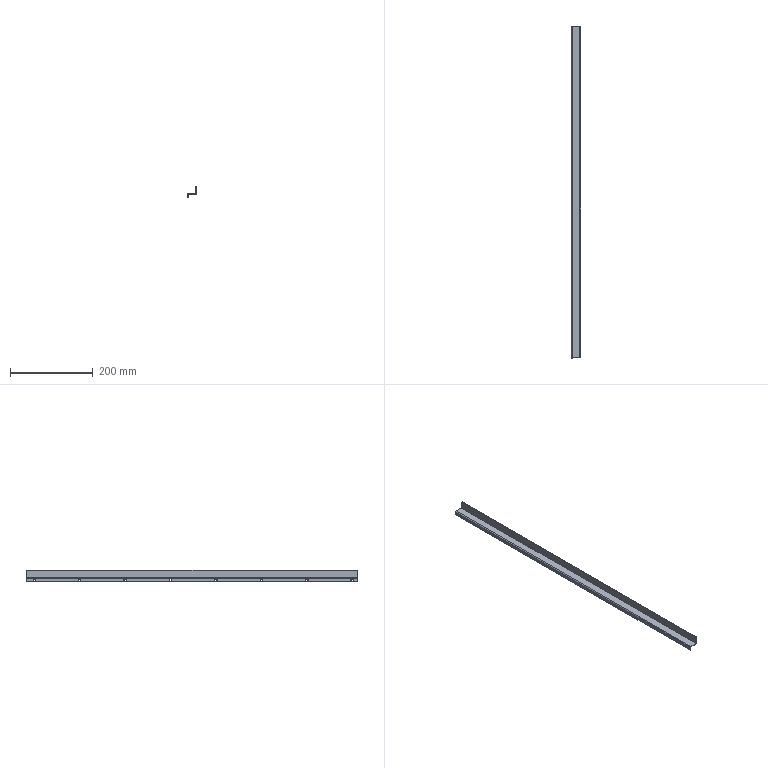Part | STEP file | Left Door Frame 1 | 1 solid | 38 faces | box 22 x 804 x 28 mm | volume 75069 mm3 | cylinder 22 | plane 16 | commonest cylinder face diameters 6 x16 0.2 x2 0.4 x2 4.2 x2
STEP:
#1=CARTESIAN_POINT('',(-10.939,692.193,-3.));
#2=VERTEX_POINT('',#1);
#3=CARTESIAN_POINT('',(-10.939,692.193,-9.));
#4=VERTEX_POINT('',#3);
#5=CARTESIAN_POINT('',(-10.939,692.193,-6.));
#6=DIRECTION('',(1.,0.,0.));
#7=DIRECTION('',(0.,0.,-1.));
#8=AXIS2_PLACEMENT_3D('',#5,#6,#7);
#9=CIRCLE('',#8,3.);
#10=EDGE_CURVE('',#2,#4,#9,.T.);
#11=ORIENTED_EDGE('',*,*,#10,.F.);
#12=CARTESIAN_POINT('',(-8.939,692.193,-3.));
#13=VERTEX_POINT('',#12);
#14=CARTESIAN_POINT('',(-18.939,692.193,-3.));
#15=DIRECTION('',(1.,0.,0.));
#16=VECTOR('',#15,1000.);
#17=LINE('',#14,#16);
#18=EDGE_CURVE('',#2,#13,#17,.T.);
#19=ORIENTED_EDGE('',*,*,#18,.T.);
#20=CARTESIAN_POINT('',(-8.939,692.193,-9.));
#21=VERTEX_POINT('',#20);
#22=CARTESIAN_POINT('',(-8.939,692.193,-6.));
#23=DIRECTION('',(-1.,0.,0.));
#24=DIRECTION('',(0.,0.,-1.));
#25=AXIS2_PLACEMENT_3D('',#22,#23,#24);
#26=CIRCLE('',#25,3.);
#27=EDGE_CURVE('',#21,#13,#26,.T.);
#28=ORIENTED_EDGE('',*,*,#27,.F.);
#29=CARTESIAN_POINT('',(-18.939,692.193,-9.));
#30=DIRECTION('',(1.,0.,0.));
#31=VECTOR('',#30,1000.);
#32=LINE('',#29,#31);
#33=EDGE_CURVE('',#4,#21,#32,.T.);
#34=ORIENTED_EDGE('',*,*,#33,.F.);
#35=EDGE_LOOP('',(#11,#19,#28,#34));
#36=FACE_OUTER_BOUND('',#35,.T.);
#37=CARTESIAN_POINT('',(-18.939,692.193,-6.));
#38=DIRECTION('',(1.,0.,0.));
#39=DIRECTION('',(0.,0.,-1.));
#40=AXIS2_PLACEMENT_3D('',#37,#38,#39);
#41=CYLINDRICAL_SURFACE('',#40,3.);
#42=ADVANCED_FACE('',(#36),#41,.F.);
#43=CARTESIAN_POINT('',(-10.939,582.193,-3.));
#44=VERTEX_POINT('',#43);
#45=CARTESIAN_POINT('',(-10.939,582.193,-9.));
#46=VERTEX_POINT('',#45);
#47=CARTESIAN_POINT('',(-10.939,582.193,-6.));
#48=DIRECTION('',(1.,0.,0.));
#49=DIRECTION('',(0.,0.,-1.));
#50=AXIS2_PLACEMENT_3D('',#47,#48,#49);
#51=CIRCLE('',#50,3.);
#52=EDGE_CURVE('',#44,#46,#51,.T.);
#53=ORIENTED_EDGE('',*,*,#52,.F.);
#54=CARTESIAN_POINT('',(-8.939,582.193,-3.));
#55=VERTEX_POINT('',#54);
#56=CARTESIAN_POINT('',(-18.939,582.193,-3.));
#57=DIRECTION('',(1.,0.,0.));
#58=VECTOR('',#57,1000.);
#59=LINE('',#56,#58);
#60=EDGE_CURVE('',#44,#55,#59,.T.);
#61=ORIENTED_EDGE('',*,*,#60,.T.);
#62=CARTESIAN_POINT('',(-8.939,582.193,-9.));
#63=VERTEX_POINT('',#62);
#64=CARTESIAN_POINT('',(-8.939,582.193,-6.));
#65=DIRECTION('',(-1.,0.,0.));
#66=DIRECTION('',(0.,0.,-1.));
#67=AXIS2_PLACEMENT_3D('',#64,#65,#66);
#68=CIRCLE('',#67,3.);
#69=EDGE_CURVE('',#63,#55,#68,.T.);
#70=ORIENTED_EDGE('',*,*,#69,.F.);
#71=CARTESIAN_POINT('',(-18.939,582.193,-9.));
#72=DIRECTION('',(1.,0.,0.));
#73=VECTOR('',#72,1000.);
#74=LINE('',#71,#73);
#75=EDGE_CURVE('',#46,#63,#74,.T.);
#76=ORIENTED_EDGE('',*,*,#75,.F.);
#77=EDGE_LOOP('',(#53,#61,#70,#76));
#78=FACE_OUTER_BOUND('',#77,.T.);
#79=CARTESIAN_POINT('',(-18.939,582.193,-6.));
#80=DIRECTION('',(1.,0.,0.));
#81=DIRECTION('',(0.,0.,-1.));
#82=AXIS2_PLACEMENT_3D('',#79,#80,#81);
#83=CYLINDRICAL_SURFACE('',#82,3.);
#84=ADVANCED_FACE('',(#78),#83,.F.);
#85=CARTESIAN_POINT('',(-10.939,472.193,-3.));
#86=VERTEX_POINT('',#85);
#87=CARTESIAN_POINT('',(-10.939,472.193,-9.));
#88=VERTEX_POINT('',#87);
#89=CARTESIAN_POINT('',(-10.939,472.193,-6.));
#90=DIRECTION('',(1.,0.,0.));
#91=DIRECTION('',(0.,0.,-1.));
#92=AXIS2_PLACEMENT_3D('',#89,#90,#91);
#93=CIRCLE('',#92,3.);
#94=EDGE_CURVE('',#86,#88,#93,.T.);
#95=ORIENTED_EDGE('',*,*,#94,.F.);
#96=CARTESIAN_POINT('',(-8.939,472.193,-3.));
#97=VERTEX_POINT('',#96);
#98=CARTESIAN_POINT('',(-18.939,472.193,-3.));
#99=DIRECTION('',(1.,0.,0.));
#100=VECTOR('',#99,1000.);
#101=LINE('',#98,#100);
#102=EDGE_CURVE('',#86,#97,#101,.T.);
#103=ORIENTED_EDGE('',*,*,#102,.T.);
#104=CARTESIAN_POINT('',(-8.939,472.193,-9.));
#105=VERTEX_POINT('',#104);
#106=CARTESIAN_POINT('',(-8.939,472.193,-6.));
#107=DIRECTION('',(-1.,0.,0.));
#108=DIRECTION('',(0.,0.,-1.));
#109=AXIS2_PLACEMENT_3D('',#106,#107,#108);
#110=CIRCLE('',#109,3.);
#111=EDGE_CURVE('',#105,#97,#110,.T.);
#112=ORIENTED_EDGE('',*,*,#111,.F.);
#113=CARTESIAN_POINT('',(-18.939,472.193,-9.));
#114=DIRECTION('',(1.,0.,0.));
#115=VECTOR('',#114,1000.);
#116=LINE('',#113,#115);
#117=EDGE_CURVE('',#88,#105,#116,.T.);
#118=ORIENTED_EDGE('',*,*,#117,.F.);
#119=EDGE_LOOP('',(#95,#103,#112,#118));
#120=FACE_OUTER_BOUND('',#119,.T.);
#121=CARTESIAN_POINT('',(-18.939,472.193,-6.));
#122=DIRECTION('',(1.,0.,0.));
#123=DIRECTION('',(0.,0.,-1.));
#124=AXIS2_PLACEMENT_3D('',#121,#122,#123);
#125=CYLINDRICAL_SURFACE('',#124,3.);
#126=ADVANCED_FACE('',(#120),#125,.F.);
#127=CARTESIAN_POINT('',(-10.939,362.193,-3.));
#128=VERTEX_POINT('',#127);
#129=CARTESIAN_POINT('',(-10.939,362.193,-9.));
#130=VERTEX_POINT('',#129);
#131=CARTESIAN_POINT('',(-10.939,362.193,-6.));
#132=DIRECTION('',(1.,0.,0.));
#133=DIRECTION('',(0.,0.,-1.));
#134=AXIS2_PLACEMENT_3D('',#131,#132,#133);
#135=CIRCLE('',#134,3.);
#136=EDGE_CURVE('',#128,#130,#135,.T.);
#137=ORIENTED_EDGE('',*,*,#136,.F.);
#138=CARTESIAN_POINT('',(-8.939,362.193,-3.));
#139=VERTEX_POINT('',#138);
#140=CARTESIAN_POINT('',(-18.939,362.193,-3.));
#141=DIRECTION('',(1.,0.,0.));
#142=VECTOR('',#141,1000.);
#143=LINE('',#140,#142);
#144=EDGE_CURVE('',#128,#139,#143,.T.);
#145=ORIENTED_EDGE('',*,*,#144,.T.);
#146=CARTESIAN_POINT('',(-8.939,362.193,-9.));
#147=VERTEX_POINT('',#146);
#148=CARTESIAN_POINT('',(-8.939,362.193,-6.));
#149=DIRECTION('',(-1.,0.,0.));
#150=DIRECTION('',(0.,0.,-1.));
#151=AXIS2_PLACEMENT_3D('',#148,#149,#150);
#152=CIRCLE('',#151,3.);
#153=EDGE_CURVE('',#147,#139,#152,.T.);
#154=ORIENTED_EDGE('',*,*,#153,.F.);
#155=CARTESIAN_POINT('',(-18.939,362.193,-9.));
#156=DIRECTION('',(1.,0.,0.));
#157=VECTOR('',#156,1000.);
#158=LINE('',#155,#157);
#159=EDGE_CURVE('',#130,#147,#158,.T.);
#160=ORIENTED_EDGE('',*,*,#159,.F.);
#161=EDGE_LOOP('',(#137,#145,#154,#160));
#162=FACE_OUTER_BOUND('',#161,.T.);
#163=CARTESIAN_POINT('',(-18.939,362.193,-6.));
#164=DIRECTION('',(1.,0.,0.));
#165=DIRECTION('',(0.,0.,-1.));
#166=AXIS2_PLACEMENT_3D('',#163,#164,#165);
#167=CYLINDRICAL_SURFACE('',#166,3.);
#168=ADVANCED_FACE('',(#162),#167,.F.);
#169=CARTESIAN_POINT('',(-10.939,252.193,-3.));
#170=VERTEX_POINT('',#169);
#171=CARTESIAN_POINT('',(-10.939,252.193,-9.));
#172=VERTEX_POINT('',#171);
#173=CARTESIAN_POINT('',(-10.939,252.193,-6.));
#174=DIRECTION('',(1.,0.,0.));
#175=DIRECTION('',(0.,0.,-1.));
#176=AXIS2_PLACEMENT_3D('',#173,#174,#175);
#177=CIRCLE('',#176,3.);
#178=EDGE_CURVE('',#170,#172,#177,.T.);
#179=ORIENTED_EDGE('',*,*,#178,.F.);
#180=CARTESIAN_POINT('',(-8.939,252.193,-3.));
#181=VERTEX_POINT('',#180);
#182=CARTESIAN_POINT('',(-18.939,252.193,-3.));
#183=DIRECTION('',(1.,0.,0.));
#184=VECTOR('',#183,1000.);
#185=LINE('',#182,#184);
#186=EDGE_CURVE('',#170,#181,#185,.T.);
#187=ORIENTED_EDGE('',*,*,#186,.T.);
#188=CARTESIAN_POINT('',(-8.939,252.193,-9.));
#189=VERTEX_POINT('',#188);
#190=CARTESIAN_POINT('',(-8.939,252.193,-6.));
#191=DIRECTION('',(-1.,0.,0.));
#192=DIRECTION('',(0.,0.,-1.));
#193=AXIS2_PLACEMENT_3D('',#190,#191,#192);
#194=CIRCLE('',#193,3.);
#195=EDGE_CURVE('',#189,#181,#194,.T.);
#196=ORIENTED_EDGE('',*,*,#195,.F.);
#197=CARTESIAN_POINT('',(-18.939,252.193,-9.));
#198=DIRECTION('',(1.,0.,0.));
#199=VECTOR('',#198,1000.);
#200=LINE('',#197,#199);
#201=EDGE_CURVE('',#172,#189,#200,.T.);
#202=ORIENTED_EDGE('',*,*,#201,.F.);
#203=EDGE_LOOP('',(#179,#187,#196,#202));
#204=FACE_OUTER_BOUND('',#203,.T.);
#205=CARTESIAN_POINT('',(-18.939,252.193,-6.));
#206=DIRECTION('',(1.,0.,0.));
#207=DIRECTION('',(0.,0.,-1.));
#208=AXIS2_PLACEMENT_3D('',#205,#206,#207);
#209=CYLINDRICAL_SURFACE('',#208,3.);
#210=ADVANCED_FACE('',(#204),#209,.F.);
#211=CARTESIAN_POINT('',(-10.939,142.193,-3.));
#212=VERTEX_POINT('',#211);
#213=CARTESIAN_POINT('',(-10.939,142.193,-9.));
#214=VERTEX_POINT('',#213);
#215=CARTESIAN_POINT('',(-10.939,142.193,-6.));
#216=DIRECTION('',(1.,0.,0.));
#217=DIRECTION('',(0.,0.,-1.));
#218=AXIS2_PLACEMENT_3D('',#215,#216,#217);
#219=CIRCLE('',#218,3.);
#220=EDGE_CURVE('',#212,#214,#219,.T.);
#221=ORIENTED_EDGE('',*,*,#220,.F.);
#222=CARTESIAN_POINT('',(-8.939,142.193,-3.));
#223=VERTEX_POINT('',#222);
#224=CARTESIAN_POINT('',(-18.939,142.193,-3.));
#225=DIRECTION('',(1.,0.,0.));
#226=VECTOR('',#225,1000.);
#227=LINE('',#224,#226);
#228=EDGE_CURVE('',#212,#223,#227,.T.);
#229=ORIENTED_EDGE('',*,*,#228,.T.);
#230=CARTESIAN_POINT('',(-8.939,142.193,-9.));
#231=VERTEX_POINT('',#230);
#232=CARTESIAN_POINT('',(-8.939,142.193,-6.));
#233=DIRECTION('',(-1.,0.,0.));
#234=DIRECTION('',(0.,0.,-1.));
#235=AXIS2_PLACEMENT_3D('',#232,#233,#234);
#236=CIRCLE('',#235,3.);
#237=EDGE_CURVE('',#231,#223,#236,.T.);
#238=ORIENTED_EDGE('',*,*,#237,.F.);
#239=CARTESIAN_POINT('',(-18.939,142.193,-9.));
#240=DIRECTION('',(1.,0.,0.));
#241=VECTOR('',#240,1000.);
#242=LINE('',#239,#241);
#243=EDGE_CURVE('',#214,#231,#242,.T.);
#244=ORIENTED_EDGE('',*,*,#243,.F.);
#245=EDGE_LOOP('',(#221,#229,#238,#244));
#246=FACE_OUTER_BOUND('',#245,.T.);
#247=CARTESIAN_POINT('',(-18.939,142.193,-6.));
#248=DIRECTION('',(1.,0.,0.));
#249=DIRECTION('',(0.,0.,-1.));
#250=AXIS2_PLACEMENT_3D('',#247,#248,#249);
#251=CYLINDRICAL_SURFACE('',#250,3.);
#252=ADVANCED_FACE('',(#246),#251,.F.);
#253=CARTESIAN_POINT('',(-10.939,32.193,-3.));
#254=VERTEX_POINT('',#253);
#255=CARTESIAN_POINT('',(-10.939,32.193,-9.));
#256=VERTEX_POINT('',#255);
#257=CARTESIAN_POINT('',(-10.939,32.193,-6.));
#258=DIRECTION('',(1.,0.,0.));
#259=DIRECTION('',(0.,0.,-1.));
#260=AXIS2_PLACEMENT_3D('',#257,#258,#259);
#261=CIRCLE('',#260,3.);
#262=EDGE_CURVE('',#254,#256,#261,.T.);
#263=ORIENTED_EDGE('',*,*,#262,.F.);
#264=CARTESIAN_POINT('',(-8.939,32.193,-3.));
#265=VERTEX_POINT('',#264);
#266=CARTESIAN_POINT('',(-18.939,32.193,-3.));
#267=DIRECTION('',(1.,0.,0.));
#268=VECTOR('',#267,1000.);
#269=LINE('',#266,#268);
#270=EDGE_CURVE('',#254,#265,#269,.T.);
#271=ORIENTED_EDGE('',*,*,#270,.T.);
#272=CARTESIAN_POINT('',(-8.939,32.193,-9.));
#273=VERTEX_POINT('',#272);
#274=CARTESIAN_POINT('',(-8.939,32.193,-6.));
#275=DIRECTION('',(-1.,0.,0.));
#276=DIRECTION('',(0.,0.,-1.));
#277=AXIS2_PLACEMENT_3D('',#274,#275,#276);
#278=CIRCLE('',#277,3.);
#279=EDGE_CURVE('',#273,#265,#278,.T.);
#280=ORIENTED_EDGE('',*,*,#279,.F.);
#281=CARTESIAN_POINT('',(-18.939,32.193,-9.));
#282=DIRECTION('',(1.,0.,0.));
#283=VECTOR('',#282,1000.);
#284=LINE('',#281,#283);
#285=EDGE_CURVE('',#256,#273,#284,.T.);
#286=ORIENTED_EDGE('',*,*,#285,.F.);
#287=EDGE_LOOP('',(#263,#271,#280,#286));
#288=FACE_OUTER_BOUND('',#287,.T.);
#289=CARTESIAN_POINT('',(-18.939,32.193,-6.));
#290=DIRECTION('',(1.,0.,0.));
#291=DIRECTION('',(0.,0.,-1.));
#292=AXIS2_PLACEMENT_3D('',#289,#290,#291);
#293=CYLINDRICAL_SURFACE('',#292,3.);
#294=ADVANCED_FACE('',(#288),#293,.F.);
#295=CARTESIAN_POINT('',(-10.939,-77.807,-3.));
#296=VERTEX_POINT('',#295);
#297=CARTESIAN_POINT('',(-10.939,-77.807,-9.));
#298=VERTEX_POINT('',#297);
#299=CARTESIAN_POINT('',(-10.939,-77.807,-6.));
#300=DIRECTION('',(1.,0.,0.));
#301=DIRECTION('',(0.,0.,-1.));
#302=AXIS2_PLACEMENT_3D('',#299,#300,#301);
#303=CIRCLE('',#302,3.);
#304=EDGE_CURVE('',#296,#298,#303,.T.);
#305=ORIENTED_EDGE('',*,*,#304,.F.);
#306=CARTESIAN_POINT('',(-8.939,-77.807,-3.));
#307=VERTEX_POINT('',#306);
#308=CARTESIAN_POINT('',(-18.939,-77.807,-3.));
#309=DIRECTION('',(1.,0.,0.));
#310=VECTOR('',#309,1000.);
#311=LINE('',#308,#310);
#312=EDGE_CURVE('',#296,#307,#311,.T.);
#313=ORIENTED_EDGE('',*,*,#312,.T.);
#314=CARTESIAN_POINT('',(-8.939,-77.807,-9.));
#315=VERTEX_POINT('',#314);
#316=CARTESIAN_POINT('',(-8.939,-77.807,-6.));
#317=DIRECTION('',(-1.,0.,0.));
#318=DIRECTION('',(0.,0.,-1.));
#319=AXIS2_PLACEMENT_3D('',#316,#317,#318);
#320=CIRCLE('',#319,3.);
#321=EDGE_CURVE('',#315,#307,#320,.T.);
#322=ORIENTED_EDGE('',*,*,#321,.F.);
#323=CARTESIAN_POINT('',(-18.939,-77.807,-9.));
#324=DIRECTION('',(1.,0.,0.));
#325=VECTOR('',#324,1000.);
#326=LINE('',#323,#325);
#327=EDGE_CURVE('',#298,#315,#326,.T.);
#328=ORIENTED_EDGE('',*,*,#327,.F.);
#329=EDGE_LOOP('',(#305,#313,#322,#328));
#330=FACE_OUTER_BOUND('',#329,.T.);
#331=CARTESIAN_POINT('',(-18.939,-77.807,-6.));
#332=DIRECTION('',(1.,0.,0.));
#333=DIRECTION('',(0.,0.,-1.));
#334=AXIS2_PLACEMENT_3D('',#331,#332,#333);
#335=CYLINDRICAL_SURFACE('',#334,3.);
#336=ADVANCED_FACE('',(#330),#335,.F.);
#337=CARTESIAN_POINT('',(9.061,-89.807,0.1));
#338=VERTEX_POINT('',#337);
#339=CARTESIAN_POINT('',(9.061,-89.807,18.));
#340=VERTEX_POINT('',#339);
#341=CARTESIAN_POINT('',(9.061,-89.807,0.));
#342=DIRECTION('',(0.,0.,1.));
#343=VECTOR('',#342,1000.);
#344=LINE('',#341,#343);
#345=EDGE_CURVE('',#338,#340,#344,.T.);
#346=ORIENTED_EDGE('',*,*,#345,.T.);
#347=CARTESIAN_POINT('',(9.061,710.193,18.));
#348=VERTEX_POINT('',#347);
#349=CARTESIAN_POINT('',(9.061,0.,18.));
#350=DIRECTION('',(0.,1.,0.));
#351=VECTOR('',#350,1000.);
#352=LINE('',#349,#351);
#353=EDGE_CURVE('',#340,#348,#352,.T.);
#354=ORIENTED_EDGE('',*,*,#353,.T.);
#355=CARTESIAN_POINT('',(9.061,710.193,0.1));
#356=VERTEX_POINT('',#355);
#357=CARTESIAN_POINT('',(9.061,710.193,0.));
#358=DIRECTION('',(0.,0.,-1.));
#359=VECTOR('',#358,1000.);
#360=LINE('',#357,#359);
#361=EDGE_CURVE('',#348,#356,#360,.T.);
#362=ORIENTED_EDGE('',*,*,#361,.T.);
#363=CARTESIAN_POINT('',(9.061,0.,0.1));
#364=DIRECTION('',(0.,-1.,0.));
#365=VECTOR('',#364,1000.);
#366=LINE('',#363,#365);
#367=EDGE_CURVE('',#356,#338,#366,.T.);
#368=ORIENTED_EDGE('',*,*,#367,.T.);
#369=EDGE_LOOP('',(#346,#354,#362,#368));
#370=FACE_OUTER_BOUND('',#369,.T.);
#371=CARTESIAN_POINT('',(9.061,0.,0.));
#372=DIRECTION('',(-1.,0.,0.));
#373=DIRECTION('',(0.,0.,1.));
#374=AXIS2_PLACEMENT_3D('',#371,#372,#373);
#375=PLANE('',#374);
#376=ADVANCED_FACE('',(#370),#375,.T.);
#377=CARTESIAN_POINT('',(11.061,-89.807,18.));
#378=VERTEX_POINT('',#377);
#379=CARTESIAN_POINT('',(11.061,-89.807,18.));
#380=DIRECTION('',(-1.,0.,0.));
#381=VECTOR('',#380,1000.);
#382=LINE('',#379,#381);
#383=EDGE_CURVE('',#378,#340,#382,.T.);
#384=ORIENTED_EDGE('',*,*,#383,.F.);
#385=CARTESIAN_POINT('',(11.061,710.193,18.));
#386=VERTEX_POINT('',#385);
#387=CARTESIAN_POINT('',(11.061,-89.807,18.));
#388=DIRECTION('',(0.,-1.,0.));
#389=VECTOR('',#388,1000.);
#390=LINE('',#387,#389);
#391=EDGE_CURVE('',#386,#378,#390,.T.);
#392=ORIENTED_EDGE('',*,*,#391,.F.);
#393=CARTESIAN_POINT('',(11.061,710.193,18.));
#394=DIRECTION('',(1.,0.,0.));
#395=VECTOR('',#394,1000.);
#396=LINE('',#393,#395);
#397=EDGE_CURVE('',#348,#386,#396,.T.);
#398=ORIENTED_EDGE('',*,*,#397,.F.);
#399=ORIENTED_EDGE('',*,*,#353,.F.);
#400=EDGE_LOOP('',(#384,#392,#398,#399));
#401=FACE_OUTER_BOUND('',#400,.T.);
#402=CARTESIAN_POINT('',(11.061,-89.807,18.));
#403=DIRECTION('',(0.,0.,-1.));
#404=DIRECTION('',(-1.,0.,0.));
#405=AXIS2_PLACEMENT_3D('',#402,#403,#404);
#406=PLANE('',#405);
#407=ADVANCED_FACE('',(#401),#406,.F.);
#408=CARTESIAN_POINT('',(11.061,-89.807,0.1));
#409=VERTEX_POINT('',#408);
#410=CARTESIAN_POINT('',(11.061,-89.807,0.));
#411=DIRECTION('',(0.,0.,-1.));
#412=VECTOR('',#411,1000.);
#413=LINE('',#410,#412);
#414=EDGE_CURVE('',#378,#409,#413,.T.);
#415=ORIENTED_EDGE('',*,*,#414,.F.);
#416=ORIENTED_EDGE('',*,*,#383,.T.);
#417=ORIENTED_EDGE('',*,*,#345,.F.);
#418=CARTESIAN_POINT('',(8.961,-89.807,0.));
#419=VERTEX_POINT('',#418);
#420=CARTESIAN_POINT('',(8.961,-89.807,0.1));
#421=DIRECTION('',(0.,1.,0.));
#422=DIRECTION('',(0.,0.,1.));
#423=AXIS2_PLACEMENT_3D('',#420,#421,#422);
#424=CIRCLE('',#423,0.1);
#425=EDGE_CURVE('',#338,#419,#424,.T.);
#426=ORIENTED_EDGE('',*,*,#425,.T.);
#427=CARTESIAN_POINT('',(8.561,-89.807,0.));
#428=VERTEX_POINT('',#427);
#429=CARTESIAN_POINT('',(0.,-89.807,0.));
#430=DIRECTION('',(1.,0.,0.));
#431=VECTOR('',#430,1000.);
#432=LINE('',#429,#431);
#433=EDGE_CURVE('',#428,#419,#432,.T.);
#434=ORIENTED_EDGE('',*,*,#433,.F.);
#435=CARTESIAN_POINT('',(8.561,-89.807,-2.));
#436=VERTEX_POINT('',#435);
#437=CARTESIAN_POINT('',(8.561,-89.807,0.));
#438=DIRECTION('',(0.,0.,-1.));
#439=VECTOR('',#438,1000.);
#440=LINE('',#437,#439);
#441=EDGE_CURVE('',#428,#436,#440,.T.);
#442=ORIENTED_EDGE('',*,*,#441,.T.);
#443=CARTESIAN_POINT('',(8.961,-89.807,-2.));
#444=VERTEX_POINT('',#443);
#445=CARTESIAN_POINT('',(8.961,-89.807,-2.));
#446=DIRECTION('',(1.,0.,0.));
#447=VECTOR('',#446,1000.);
#448=LINE('',#445,#447);
#449=EDGE_CURVE('',#436,#444,#448,.T.);
#450=ORIENTED_EDGE('',*,*,#449,.T.);
#451=CARTESIAN_POINT('',(8.961,-89.807,0.1));
#452=DIRECTION('',(0.,-1.,0.));
#453=DIRECTION('',(0.,0.,1.));
#454=AXIS2_PLACEMENT_3D('',#451,#452,#453);
#455=CIRCLE('',#454,2.1);
#456=EDGE_CURVE('',#444,#409,#455,.T.);
#457=ORIENTED_EDGE('',*,*,#456,.T.);
#458=EDGE_LOOP('',(#415,#416,#417,#426,#434,#442,#450,#457));
#459=FACE_OUTER_BOUND('',#458,.T.);
#460=CARTESIAN_POINT('',(11.061,-89.807,0.));
#461=DIRECTION('',(0.,1.,0.));
#462=DIRECTION('',(-1.,0.,0.));
#463=AXIS2_PLACEMENT_3D('',#460,#461,#462);
#464=PLANE('',#463);
#465=ADVANCED_FACE('',(#459),#464,.F.);
#466=ORIENTED_EDGE('',*,*,#425,.F.);
#467=ORIENTED_EDGE('',*,*,#367,.F.);
#468=CARTESIAN_POINT('',(8.961,710.193,0.));
#469=VERTEX_POINT('',#468);
#470=CARTESIAN_POINT('',(8.961,710.193,0.1));
#471=DIRECTION('',(0.,1.,0.));
#472=DIRECTION('',(0.,0.,1.));
#473=AXIS2_PLACEMENT_3D('',#470,#471,#472);
#474=CIRCLE('',#473,0.1);
#475=EDGE_CURVE('',#356,#469,#474,.T.);
#476=ORIENTED_EDGE('',*,*,#475,.T.);
#477=CARTESIAN_POINT('',(8.961,710.193,0.));
#478=DIRECTION('',(0.,1.,0.));
#479=VECTOR('',#478,1000.);
#480=LINE('',#477,#479);
#481=EDGE_CURVE('',#419,#469,#480,.T.);
#482=ORIENTED_EDGE('',*,*,#481,.F.);
#483=EDGE_LOOP('',(#466,#467,#476,#482));
#484=FACE_OUTER_BOUND('',#483,.T.);
#485=CARTESIAN_POINT('',(8.961,710.193,0.1));
#486=DIRECTION('',(0.,1.,0.));
#487=DIRECTION('',(0.,0.,1.));
#488=AXIS2_PLACEMENT_3D('',#485,#486,#487);
#489=CYLINDRICAL_SURFACE('',#488,0.1);
#490=ADVANCED_FACE('',(#484),#489,.F.);
#491=ORIENTED_EDGE('',*,*,#361,.F.);
#492=ORIENTED_EDGE('',*,*,#397,.T.);
#493=CARTESIAN_POINT('',(11.061,710.193,0.1));
#494=VERTEX_POINT('',#493);
#495=CARTESIAN_POINT('',(11.061,710.193,18.));
#496=DIRECTION('',(0.,0.,1.));
#497=VECTOR('',#496,1000.);
#498=LINE('',#495,#497);
#499=EDGE_CURVE('',#494,#386,#498,.T.);
#500=ORIENTED_EDGE('',*,*,#499,.F.);
#501=CARTESIAN_POINT('',(8.961,710.193,-2.));
#502=VERTEX_POINT('',#501);
#503=CARTESIAN_POINT('',(8.961,710.193,0.1));
#504=DIRECTION('',(0.,-1.,0.));
#505=DIRECTION('',(0.,0.,1.));
#506=AXIS2_PLACEMENT_3D('',#503,#504,#505);
#507=CIRCLE('',#506,2.1);
#508=EDGE_CURVE('',#502,#494,#507,.T.);
#509=ORIENTED_EDGE('',*,*,#508,.F.);
#510=CARTESIAN_POINT('',(8.561,710.193,-2.));
#511=VERTEX_POINT('',#510);
#512=CARTESIAN_POINT('',(8.561,710.193,-2.));
#513=DIRECTION('',(-1.,0.,0.));
#514=VECTOR('',#513,1000.);
#515=LINE('',#512,#514);
#516=EDGE_CURVE('',#502,#511,#515,.T.);
#517=ORIENTED_EDGE('',*,*,#516,.T.);
#518=CARTESIAN_POINT('',(8.561,710.193,0.));
#519=VERTEX_POINT('',#518);
#520=CARTESIAN_POINT('',(8.561,710.193,0.));
#521=DIRECTION('',(0.,0.,1.));
#522=VECTOR('',#521,1000.);
#523=LINE('',#520,#522);
#524=EDGE_CURVE('',#511,#519,#523,.T.);
#525=ORIENTED_EDGE('',*,*,#524,.T.);
#526=CARTESIAN_POINT('',(8.561,710.193,0.));
#527=DIRECTION('',(1.,0.,0.));
#528=VECTOR('',#527,1000.);
#529=LINE('',#526,#528);
#530=EDGE_CURVE('',#519,#469,#529,.T.);
#531=ORIENTED_EDGE('',*,*,#530,.T.);
#532=ORIENTED_EDGE('',*,*,#475,.F.);
#533=EDGE_LOOP('',(#491,#492,#500,#509,#517,#525,#531,#532));
#534=FACE_OUTER_BOUND('',#533,.T.);
#535=CARTESIAN_POINT('',(11.061,710.193,18.));
#536=DIRECTION('',(0.,-1.,0.));
#537=DIRECTION('',(1.,0.,0.));
#538=AXIS2_PLACEMENT_3D('',#535,#536,#537);
#539=PLANE('',#538);
#540=ADVANCED_FACE('',(#534),#539,.F.);
#541=ORIENTED_EDGE('',*,*,#499,.T.);
#542=ORIENTED_EDGE('',*,*,#391,.T.);
#543=ORIENTED_EDGE('',*,*,#414,.T.);
#544=CARTESIAN_POINT('',(11.061,0.,0.1));
#545=DIRECTION('',(0.,-1.,0.));
#546=VECTOR('',#545,1000.);
#547=LINE('',#544,#546);
#548=EDGE_CURVE('',#494,#409,#547,.T.);
#549=ORIENTED_EDGE('',*,*,#548,.F.);
#550=EDGE_LOOP('',(#541,#542,#543,#549));
#551=FACE_OUTER_BOUND('',#550,.T.);
#552=CARTESIAN_POINT('',(11.061,0.,0.));
#553=DIRECTION('',(-1.,0.,0.));
#554=DIRECTION('',(0.,0.,1.));
#555=AXIS2_PLACEMENT_3D('',#552,#553,#554);
#556=PLANE('',#555);
#557=ADVANCED_FACE('',(#551),#556,.F.);
#558=ORIENTED_EDGE('',*,*,#481,.T.);
#559=ORIENTED_EDGE('',*,*,#530,.F.);
#560=CARTESIAN_POINT('',(8.561,710.593,0.));
#561=VERTEX_POINT('',#560);
#562=CARTESIAN_POINT('',(8.561,710.393,0.));
#563=DIRECTION('',(0.,0.,-1.));
#564=DIRECTION('',(0.,1.,0.));
#565=AXIS2_PLACEMENT_3D('',#562,#563,#564);
#566=CIRCLE('',#565,0.2);
#567=EDGE_CURVE('',#519,#561,#566,.T.);
#568=ORIENTED_EDGE('',*,*,#567,.T.);
#569=CARTESIAN_POINT('',(11.061,710.593,0.));
#570=VERTEX_POINT('',#569);
#571=CARTESIAN_POINT('',(0.,710.593,0.));
#572=DIRECTION('',(1.,0.,0.));
#573=VECTOR('',#572,1000.);
#574=LINE('',#571,#573);
#575=EDGE_CURVE('',#561,#570,#574,.T.);
#576=ORIENTED_EDGE('',*,*,#575,.T.);
#577=CARTESIAN_POINT('',(11.061,712.193,0.));
#578=VERTEX_POINT('',#577);
#579=CARTESIAN_POINT('',(11.061,712.193,0.));
#580=DIRECTION('',(0.,-1.,0.));
#581=VECTOR('',#580,1000.);
#582=LINE('',#579,#581);
#583=EDGE_CURVE('',#578,#570,#582,.T.);
#584=ORIENTED_EDGE('',*,*,#583,.F.);
#585=CARTESIAN_POINT('',(-8.839,712.193,0.));
#586=VERTEX_POINT('',#585);
#587=CARTESIAN_POINT('',(0.,712.193,0.));
#588=DIRECTION('',(-1.,0.,0.));
#589=VECTOR('',#588,1000.);
#590=LINE('',#587,#589);
#591=EDGE_CURVE('',#578,#586,#590,.T.);
#592=ORIENTED_EDGE('',*,*,#591,.T.);
#593=CARTESIAN_POINT('',(-8.839,-91.807,0.));
#594=VERTEX_POINT('',#593);
#595=CARTESIAN_POINT('',(-8.839,0.,0.));
#596=DIRECTION('',(0.,-1.,0.));
#597=VECTOR('',#596,1000.);
#598=LINE('',#595,#597);
#599=EDGE_CURVE('',#586,#594,#598,.T.);
#600=ORIENTED_EDGE('',*,*,#599,.T.);
#601=CARTESIAN_POINT('',(11.061,-91.807,0.));
#602=VERTEX_POINT('',#601);
#603=CARTESIAN_POINT('',(0.,-91.807,0.));
#604=DIRECTION('',(1.,0.,0.));
#605=VECTOR('',#604,1000.);
#606=LINE('',#603,#605);
#607=EDGE_CURVE('',#594,#602,#606,.T.);
#608=ORIENTED_EDGE('',*,*,#607,.T.);
#609=CARTESIAN_POINT('',(11.061,-90.207,0.));
#610=VERTEX_POINT('',#609);
#611=CARTESIAN_POINT('',(11.061,712.193,0.));
#612=DIRECTION('',(0.,-1.,0.));
#613=VECTOR('',#612,1000.);
#614=LINE('',#611,#613);
#615=EDGE_CURVE('',#610,#602,#614,.T.);
#616=ORIENTED_EDGE('',*,*,#615,.F.);
#617=CARTESIAN_POINT('',(8.561,-90.207,0.));
#618=VERTEX_POINT('',#617);
#619=CARTESIAN_POINT('',(0.,-90.207,0.));
#620=DIRECTION('',(-1.,0.,0.));
#621=VECTOR('',#620,1000.);
#622=LINE('',#619,#621);
#623=EDGE_CURVE('',#610,#618,#622,.T.);
#624=ORIENTED_EDGE('',*,*,#623,.T.);
#625=CARTESIAN_POINT('',(8.561,-90.007,0.));
#626=DIRECTION('',(0.,0.,-1.));
#627=DIRECTION('',(0.,1.,0.));
#628=AXIS2_PLACEMENT_3D('',#625,#626,#627);
#629=CIRCLE('',#628,0.2);
#630=EDGE_CURVE('',#618,#428,#629,.T.);
#631=ORIENTED_EDGE('',*,*,#630,.T.);
#632=ORIENTED_EDGE('',*,*,#433,.T.);
#633=EDGE_LOOP('',(#558,#559,#568,#576,#584,#592,#600,#608,#616,#624,#631,#632));
#634=FACE_OUTER_BOUND('',#633,.T.);
#635=CARTESIAN_POINT('',(0.,0.,0.));
#636=DIRECTION('',(0.,0.,1.));
#637=DIRECTION('',(1.,0.,0.));
#638=AXIS2_PLACEMENT_3D('',#635,#636,#637);
#639=PLANE('',#638);
#640=ADVANCED_FACE('',(#634),#639,.T.);
#641=ORIENTED_EDGE('',*,*,#548,.T.);
#642=ORIENTED_EDGE('',*,*,#456,.F.);
#643=CARTESIAN_POINT('',(8.961,710.193,-2.));
#644=DIRECTION('',(0.,1.,0.));
#645=VECTOR('',#644,1000.);
#646=LINE('',#643,#645);
#647=EDGE_CURVE('',#444,#502,#646,.T.);
#648=ORIENTED_EDGE('',*,*,#647,.T.);
#649=ORIENTED_EDGE('',*,*,#508,.T.);
#650=EDGE_LOOP('',(#641,#642,#648,#649));
#651=FACE_OUTER_BOUND('',#650,.T.);
#652=CARTESIAN_POINT('',(8.961,710.193,0.1));
#653=DIRECTION('',(0.,1.,0.));
#654=DIRECTION('',(0.,0.,1.));
#655=AXIS2_PLACEMENT_3D('',#652,#653,#654);
#656=CYLINDRICAL_SURFACE('',#655,2.1);
#657=ADVANCED_FACE('',(#651),#656,.T.);
#658=CARTESIAN_POINT('',(8.561,-90.207,-2.));
#659=VERTEX_POINT('',#658);
#660=CARTESIAN_POINT('',(8.561,-90.207,0.));
#661=DIRECTION('',(0.,0.,1.));
#662=VECTOR('',#661,1000.);
#663=LINE('',#660,#662);
#664=EDGE_CURVE('',#659,#618,#663,.T.);
#665=ORIENTED_EDGE('',*,*,#664,.T.);
#666=ORIENTED_EDGE('',*,*,#623,.F.);
#667=CARTESIAN_POINT('',(11.061,-90.207,-2.));
#668=VERTEX_POINT('',#667);
#669=CARTESIAN_POINT('',(11.061,-90.207,0.));
#670=DIRECTION('',(0.,0.,-1.));
#671=VECTOR('',#670,1000.);
#672=LINE('',#669,#671);
#673=EDGE_CURVE('',#610,#668,#672,.T.);
#674=ORIENTED_EDGE('',*,*,#673,.T.);
#675=CARTESIAN_POINT('',(8.561,-90.207,-2.));
#676=DIRECTION('',(-1.,0.,0.));
#677=VECTOR('',#676,1000.);
#678=LINE('',#675,#677);
#679=EDGE_CURVE('',#668,#659,#678,.T.);
#680=ORIENTED_EDGE('',*,*,#679,.T.);
#681=EDGE_LOOP('',(#665,#666,#674,#680));
#682=FACE_OUTER_BOUND('',#681,.T.);
#683=CARTESIAN_POINT('',(8.561,-90.207,0.));
#684=DIRECTION('',(0.,1.,0.));
#685=DIRECTION('',(0.,0.,1.));
#686=AXIS2_PLACEMENT_3D('',#683,#684,#685);
#687=PLANE('',#686);
#688=ADVANCED_FACE('',(#682),#687,.T.);
#689=CARTESIAN_POINT('',(11.061,-91.807,-2.));
#690=VERTEX_POINT('',#689);
#691=CARTESIAN_POINT('',(11.061,-91.807,-2.));
#692=DIRECTION('',(0.,0.,1.));
#693=VECTOR('',#692,1000.);
#694=LINE('',#691,#693);
#695=EDGE_CURVE('',#690,#602,#694,.T.);
#696=ORIENTED_EDGE('',*,*,#695,.T.);
#697=ORIENTED_EDGE('',*,*,#607,.F.);
#698=CARTESIAN_POINT('',(-10.939,-91.807,-2.1));
#699=VERTEX_POINT('',#698);
#700=CARTESIAN_POINT('',(-8.839,-91.807,-2.1));
#701=DIRECTION('',(0.,1.,0.));
#702=DIRECTION('',(0.,0.,1.));
#703=AXIS2_PLACEMENT_3D('',#700,#701,#702);
#704=CIRCLE('',#703,2.1);
#705=EDGE_CURVE('',#699,#594,#704,.T.);
#706=ORIENTED_EDGE('',*,*,#705,.F.);
#707=CARTESIAN_POINT('',(-10.939,-91.807,-10.));
#708=VERTEX_POINT('',#707);
#709=CARTESIAN_POINT('',(-10.939,-91.807,0.));
#710=DIRECTION('',(0.,0.,1.));
#711=VECTOR('',#710,1000.);
#712=LINE('',#709,#711);
#713=EDGE_CURVE('',#708,#699,#712,.T.);
#714=ORIENTED_EDGE('',*,*,#713,.F.);
#715=CARTESIAN_POINT('',(-8.939,-91.807,-10.));
#716=VERTEX_POINT('',#715);
#717=CARTESIAN_POINT('',(-10.939,-91.807,-10.));
#718=DIRECTION('',(1.,0.,0.));
#719=VECTOR('',#718,1000.);
#720=LINE('',#717,#719);
#721=EDGE_CURVE('',#708,#716,#720,.T.);
#722=ORIENTED_EDGE('',*,*,#721,.T.);
#723=CARTESIAN_POINT('',(-8.939,-91.807,-2.1));
#724=VERTEX_POINT('',#723);
#725=CARTESIAN_POINT('',(-8.939,-91.807,-10.));
#726=DIRECTION('',(0.,0.,1.));
#727=VECTOR('',#726,1000.);
#728=LINE('',#725,#727);
#729=EDGE_CURVE('',#716,#724,#728,.T.);
#730=ORIENTED_EDGE('',*,*,#729,.T.);
#731=CARTESIAN_POINT('',(-8.839,-91.807,-2.));
#732=VERTEX_POINT('',#731);
#733=CARTESIAN_POINT('',(-8.839,-91.807,-2.1));
#734=DIRECTION('',(0.,1.,0.));
#735=DIRECTION('',(0.,0.,1.));
#736=AXIS2_PLACEMENT_3D('',#733,#734,#735);
#737=CIRCLE('',#736,0.1);
#738=EDGE_CURVE('',#724,#732,#737,.T.);
#739=ORIENTED_EDGE('',*,*,#738,.T.);
#740=CARTESIAN_POINT('',(-10.939,-91.807,-2.));
#741=DIRECTION('',(1.,0.,0.));
#742=VECTOR('',#741,1000.);
#743=LINE('',#740,#742);
#744=EDGE_CURVE('',#732,#690,#743,.T.);
#745=ORIENTED_EDGE('',*,*,#744,.T.);
#746=EDGE_LOOP('',(#696,#697,#706,#714,#722,#730,#739,#745));
#747=FACE_OUTER_BOUND('',#746,.T.);
#748=CARTESIAN_POINT('',(-10.939,-91.807,-2.));
#749=DIRECTION('',(0.,-1.,0.));
#750=DIRECTION('',(0.,0.,-1.));
#751=AXIS2_PLACEMENT_3D('',#748,#749,#750);
#752=PLANE('',#751);
#753=ADVANCED_FACE('',(#747),#752,.T.);
#754=CARTESIAN_POINT('',(-10.939,712.193,-2.1));
#755=VERTEX_POINT('',#754);
#756=CARTESIAN_POINT('',(-10.939,712.193,-2.1));
#757=DIRECTION('',(0.,-1.,0.));
#758=VECTOR('',#757,1000.);
#759=LINE('',#756,#758);
#760=EDGE_CURVE('',#755,#699,#759,.T.);
#761=ORIENTED_EDGE('',*,*,#760,.T.);
#762=ORIENTED_EDGE('',*,*,#705,.T.);
#763=ORIENTED_EDGE('',*,*,#599,.F.);
#764=CARTESIAN_POINT('',(-8.839,712.193,-2.1));
#765=DIRECTION('',(0.,-1.,0.));
#766=DIRECTION('',(0.,0.,1.));
#767=AXIS2_PLACEMENT_3D('',#764,#765,#766);
#768=CIRCLE('',#767,2.1);
#769=EDGE_CURVE('',#586,#755,#768,.T.);
#770=ORIENTED_EDGE('',*,*,#769,.T.);
#771=EDGE_LOOP('',(#761,#762,#763,#770));
#772=FACE_OUTER_BOUND('',#771,.T.);
#773=CARTESIAN_POINT('',(-8.839,712.193,-2.1));
#774=DIRECTION('',(0.,1.,0.));
#775=DIRECTION('',(0.,0.,1.));
#776=AXIS2_PLACEMENT_3D('',#773,#774,#775);
#777=CYLINDRICAL_SURFACE('',#776,2.1);
#778=ADVANCED_FACE('',(#772),#777,.T.);
#779=ORIENTED_EDGE('',*,*,#591,.F.);
#780=CARTESIAN_POINT('',(11.061,712.193,-2.));
#781=VERTEX_POINT('',#780);
#782=CARTESIAN_POINT('',(11.061,712.193,-2.));
#783=DIRECTION('',(0.,0.,-1.));
#784=VECTOR('',#783,1000.);
#785=LINE('',#782,#784);
#786=EDGE_CURVE('',#578,#781,#785,.T.);
#787=ORIENTED_EDGE('',*,*,#786,.T.);
#788=CARTESIAN_POINT('',(-8.839,712.193,-2.));
#789=VERTEX_POINT('',#788);
#790=CARTESIAN_POINT('',(-10.939,712.193,-2.));
#791=DIRECTION('',(-1.,0.,0.));
#792=VECTOR('',#791,1000.);
#793=LINE('',#790,#792);
#794=EDGE_CURVE('',#781,#789,#793,.T.);
#795=ORIENTED_EDGE('',*,*,#794,.T.);
#796=CARTESIAN_POINT('',(-8.939,712.193,-2.1));
#797=VERTEX_POINT('',#796);
#798=CARTESIAN_POINT('',(-8.839,712.193,-2.1));
#799=DIRECTION('',(0.,1.,0.));
#800=DIRECTION('',(0.,0.,1.));
#801=AXIS2_PLACEMENT_3D('',#798,#799,#800);
#802=CIRCLE('',#801,0.1);
#803=EDGE_CURVE('',#797,#789,#802,.T.);
#804=ORIENTED_EDGE('',*,*,#803,.F.);
#805=CARTESIAN_POINT('',(-8.939,712.193,-10.));
#806=VERTEX_POINT('',#805);
#807=CARTESIAN_POINT('',(-8.939,712.193,-2.));
#808=DIRECTION('',(0.,0.,-1.));
#809=VECTOR('',#808,1000.);
#810=LINE('',#807,#809);
#811=EDGE_CURVE('',#797,#806,#810,.T.);
#812=ORIENTED_EDGE('',*,*,#811,.T.);
#813=CARTESIAN_POINT('',(-10.939,712.193,-10.));
#814=VERTEX_POINT('',#813);
#815=CARTESIAN_POINT('',(-10.939,712.193,-10.));
#816=DIRECTION('',(1.,0.,0.));
#817=VECTOR('',#816,1000.);
#818=LINE('',#815,#817);
#819=EDGE_CURVE('',#814,#806,#818,.T.);
#820=ORIENTED_EDGE('',*,*,#819,.F.);
#821=CARTESIAN_POINT('',(-10.939,712.193,0.));
#822=DIRECTION('',(0.,0.,-1.));
#823=VECTOR('',#822,1000.);
#824=LINE('',#821,#823);
#825=EDGE_CURVE('',#755,#814,#824,.T.);
#826=ORIENTED_EDGE('',*,*,#825,.F.);
#827=ORIENTED_EDGE('',*,*,#769,.F.);
#828=EDGE_LOOP('',(#779,#787,#795,#804,#812,#820,#826,#827));
#829=FACE_OUTER_BOUND('',#828,.T.);
#830=CARTESIAN_POINT('',(-10.939,712.193,-2.));
#831=DIRECTION('',(0.,1.,0.));
#832=DIRECTION('',(0.,0.,1.));
#833=AXIS2_PLACEMENT_3D('',#830,#831,#832);
#834=PLANE('',#833);
#835=ADVANCED_FACE('',(#829),#834,.T.);
#836=CARTESIAN_POINT('',(11.061,710.593,-2.));
#837=VERTEX_POINT('',#836);
#838=CARTESIAN_POINT('',(11.061,710.593,0.));
#839=DIRECTION('',(0.,0.,1.));
#840=VECTOR('',#839,1000.);
#841=LINE('',#838,#840);
#842=EDGE_CURVE('',#837,#570,#841,.T.);
#843=ORIENTED_EDGE('',*,*,#842,.T.);
#844=ORIENTED_EDGE('',*,*,#575,.F.);
#845=CARTESIAN_POINT('',(8.561,710.593,-2.));
#846=VERTEX_POINT('',#845);
#847=CARTESIAN_POINT('',(8.561,710.593,0.));
#848=DIRECTION('',(0.,0.,-1.));
#849=VECTOR('',#848,1000.);
#850=LINE('',#847,#849);
#851=EDGE_CURVE('',#561,#846,#850,.T.);
#852=ORIENTED_EDGE('',*,*,#851,.T.);
#853=CARTESIAN_POINT('',(11.061,710.593,-2.));
#854=DIRECTION('',(1.,0.,0.));
#855=VECTOR('',#854,1000.);
#856=LINE('',#853,#855);
#857=EDGE_CURVE('',#846,#837,#856,.T.);
#858=ORIENTED_EDGE('',*,*,#857,.T.);
#859=EDGE_LOOP('',(#843,#844,#852,#858));
#860=FACE_OUTER_BOUND('',#859,.T.);
#861=CARTESIAN_POINT('',(11.061,710.593,0.));
#862=DIRECTION('',(0.,-1.,0.));
#863=DIRECTION('',(0.,0.,-1.));
#864=AXIS2_PLACEMENT_3D('',#861,#862,#863);
#865=PLANE('',#864);
#866=ADVANCED_FACE('',(#860),#865,.T.);
#867=CARTESIAN_POINT('',(8.561,710.393,-2.));
#868=DIRECTION('',(0.,0.,-1.));
#869=DIRECTION('',(0.,1.,0.));
#870=AXIS2_PLACEMENT_3D('',#867,#868,#869);
#871=CIRCLE('',#870,0.2);
#872=EDGE_CURVE('',#511,#846,#871,.T.);
#873=ORIENTED_EDGE('',*,*,#872,.F.);
#874=ORIENTED_EDGE('',*,*,#516,.F.);
#875=ORIENTED_EDGE('',*,*,#647,.F.);
#876=ORIENTED_EDGE('',*,*,#449,.F.);
#877=CARTESIAN_POINT('',(8.561,-90.007,-2.));
#878=DIRECTION('',(0.,0.,-1.));
#879=DIRECTION('',(0.,1.,0.));
#880=AXIS2_PLACEMENT_3D('',#877,#878,#879);
#881=CIRCLE('',#880,0.2);
#882=EDGE_CURVE('',#659,#436,#881,.T.);
#883=ORIENTED_EDGE('',*,*,#882,.F.);
#884=ORIENTED_EDGE('',*,*,#679,.F.);
#885=CARTESIAN_POINT('',(11.061,0.,-2.));
#886=DIRECTION('',(0.,1.,0.));
#887=VECTOR('',#886,1000.);
#888=LINE('',#885,#887);
#889=EDGE_CURVE('',#690,#668,#888,.T.);
#890=ORIENTED_EDGE('',*,*,#889,.F.);
#891=ORIENTED_EDGE('',*,*,#744,.F.);
#892=CARTESIAN_POINT('',(-8.839,0.,-2.));
#893=DIRECTION('',(0.,-1.,0.));
#894=VECTOR('',#893,1000.);
#895=LINE('',#892,#894);
#896=EDGE_CURVE('',#789,#732,#895,.T.);
#897=ORIENTED_EDGE('',*,*,#896,.F.);
#898=ORIENTED_EDGE('',*,*,#794,.F.);
#899=CARTESIAN_POINT('',(11.061,0.,-2.));
#900=DIRECTION('',(0.,1.,0.));
#901=VECTOR('',#900,1000.);
#902=LINE('',#899,#901);
#903=EDGE_CURVE('',#837,#781,#902,.T.);
#904=ORIENTED_EDGE('',*,*,#903,.F.);
#905=ORIENTED_EDGE('',*,*,#857,.F.);
#906=EDGE_LOOP('',(#873,#874,#875,#876,#883,#884,#890,#891,#897,#898,#904,#905));
#907=FACE_OUTER_BOUND('',#906,.T.);
#908=CARTESIAN_POINT('',(0.,0.,-2.));
#909=DIRECTION('',(0.,0.,1.));
#910=DIRECTION('',(1.,0.,0.));
#911=AXIS2_PLACEMENT_3D('',#908,#909,#910);
#912=PLANE('',#911);
#913=ADVANCED_FACE('',(#907),#912,.F.);
#914=ORIENTED_EDGE('',*,*,#882,.T.);
#915=ORIENTED_EDGE('',*,*,#441,.F.);
#916=ORIENTED_EDGE('',*,*,#630,.F.);
#917=ORIENTED_EDGE('',*,*,#664,.F.);
#918=EDGE_LOOP('',(#914,#915,#916,#917));
#919=FACE_OUTER_BOUND('',#918,.T.);
#920=CARTESIAN_POINT('',(8.561,-90.007,0.));
#921=DIRECTION('',(0.,0.,-1.));
#922=DIRECTION('',(0.,1.,0.));
#923=AXIS2_PLACEMENT_3D('',#920,#921,#922);
#924=CYLINDRICAL_SURFACE('',#923,0.2);
#925=ADVANCED_FACE('',(#919),#924,.F.);
#926=ORIENTED_EDGE('',*,*,#615,.T.);
#927=ORIENTED_EDGE('',*,*,#695,.F.);
#928=ORIENTED_EDGE('',*,*,#889,.T.);
#929=ORIENTED_EDGE('',*,*,#673,.F.);
#930=EDGE_LOOP('',(#926,#927,#928,#929));
#931=FACE_OUTER_BOUND('',#930,.T.);
#932=CARTESIAN_POINT('',(11.061,712.193,-2.));
#933=DIRECTION('',(1.,0.,0.));
#934=DIRECTION('',(0.,1.,0.));
#935=AXIS2_PLACEMENT_3D('',#932,#933,#934);
#936=PLANE('',#935);
#937=ADVANCED_FACE('',(#931),#936,.T.);
#938=ORIENTED_EDGE('',*,*,#825,.T.);
#939=CARTESIAN_POINT('',(-10.939,0.,-10.));
#940=DIRECTION('',(0.,-1.,0.));
#941=VECTOR('',#940,1000.);
#942=LINE('',#939,#941);
#943=EDGE_CURVE('',#814,#708,#942,.T.);
#944=ORIENTED_EDGE('',*,*,#943,.T.);
#945=ORIENTED_EDGE('',*,*,#713,.T.);
#946=ORIENTED_EDGE('',*,*,#760,.F.);
#947=EDGE_LOOP('',(#938,#944,#945,#946));
#948=FACE_OUTER_BOUND('',#947,.T.);
#949=CARTESIAN_POINT('',(-10.939,692.193,-6.));
#950=DIRECTION('',(1.,0.,0.));
#951=DIRECTION('',(0.,0.,-1.));
#952=AXIS2_PLACEMENT_3D('',#949,#950,#951);
#953=CIRCLE('',#952,3.);
#954=EDGE_CURVE('',#4,#2,#953,.T.);
#955=ORIENTED_EDGE('',*,*,#954,.T.);
#956=ORIENTED_EDGE('',*,*,#10,.T.);
#957=EDGE_LOOP('',(#955,#956));
#958=FACE_BOUND('',#957,.T.);
#959=CARTESIAN_POINT('',(-10.939,582.193,-6.));
#960=DIRECTION('',(1.,0.,0.));
#961=DIRECTION('',(0.,0.,-1.));
#962=AXIS2_PLACEMENT_3D('',#959,#960,#961);
#963=CIRCLE('',#962,3.);
#964=EDGE_CURVE('',#46,#44,#963,.T.);
#965=ORIENTED_EDGE('',*,*,#964,.T.);
#966=ORIENTED_EDGE('',*,*,#52,.T.);
#967=EDGE_LOOP('',(#965,#966));
#968=FACE_BOUND('',#967,.T.);
#969=CARTESIAN_POINT('',(-10.939,472.193,-6.));
#970=DIRECTION('',(1.,0.,0.));
#971=DIRECTION('',(0.,0.,-1.));
#972=AXIS2_PLACEMENT_3D('',#969,#970,#971);
#973=CIRCLE('',#972,3.);
#974=EDGE_CURVE('',#88,#86,#973,.T.);
#975=ORIENTED_EDGE('',*,*,#974,.T.);
#976=ORIENTED_EDGE('',*,*,#94,.T.);
#977=EDGE_LOOP('',(#975,#976));
#978=FACE_BOUND('',#977,.T.);
#979=CARTESIAN_POINT('',(-10.939,362.193,-6.));
#980=DIRECTION('',(1.,0.,0.));
#981=DIRECTION('',(0.,0.,-1.));
#982=AXIS2_PLACEMENT_3D('',#979,#980,#981);
#983=CIRCLE('',#982,3.);
#984=EDGE_CURVE('',#130,#128,#983,.T.);
#985=ORIENTED_EDGE('',*,*,#984,.T.);
#986=ORIENTED_EDGE('',*,*,#136,.T.);
#987=EDGE_LOOP('',(#985,#986));
#988=FACE_BOUND('',#987,.T.);
#989=CARTESIAN_POINT('',(-10.939,252.193,-6.));
#990=DIRECTION('',(1.,0.,0.));
#991=DIRECTION('',(0.,0.,-1.));
#992=AXIS2_PLACEMENT_3D('',#989,#990,#991);
#993=CIRCLE('',#992,3.);
#994=EDGE_CURVE('',#172,#170,#993,.T.);
#995=ORIENTED_EDGE('',*,*,#994,.T.);
#996=ORIENTED_EDGE('',*,*,#178,.T.);
#997=EDGE_LOOP('',(#995,#996));
#998=FACE_BOUND('',#997,.T.);
#999=CARTESIAN_POINT('',(-10.939,142.193,-6.));
#1000=DIRECTION('',(1.,0.,0.));
#1001=DIRECTION('',(0.,0.,-1.));
#1002=AXIS2_PLACEMENT_3D('',#999,#1000,#1001);
#1003=CIRCLE('',#1002,3.);
#1004=EDGE_CURVE('',#214,#212,#1003,.T.);
#1005=ORIENTED_EDGE('',*,*,#1004,.T.);
#1006=ORIENTED_EDGE('',*,*,#220,.T.);
#1007=EDGE_LOOP('',(#1005,#1006));
#1008=FACE_BOUND('',#1007,.T.);
#1009=CARTESIAN_POINT('',(-10.939,32.193,-6.));
#1010=DIRECTION('',(1.,0.,0.));
#1011=DIRECTION('',(0.,0.,-1.));
#1012=AXIS2_PLACEMENT_3D('',#1009,#1010,#1011);
#1013=CIRCLE('',#1012,3.);
#1014=EDGE_CURVE('',#256,#254,#1013,.T.);
#1015=ORIENTED_EDGE('',*,*,#1014,.T.);
#1016=ORIENTED_EDGE('',*,*,#262,.T.);
#1017=EDGE_LOOP('',(#1015,#1016));
#1018=FACE_BOUND('',#1017,.T.);
#1019=CARTESIAN_POINT('',(-10.939,-77.807,-6.));
#1020=DIRECTION('',(1.,0.,0.));
#1021=DIRECTION('',(0.,0.,-1.));
#1022=AXIS2_PLACEMENT_3D('',#1019,#1020,#1021);
#1023=CIRCLE('',#1022,3.);
#1024=EDGE_CURVE('',#298,#296,#1023,.T.);
#1025=ORIENTED_EDGE('',*,*,#1024,.T.);
#1026=ORIENTED_EDGE('',*,*,#304,.T.);
#1027=EDGE_LOOP('',(#1025,#1026));
#1028=FACE_BOUND('',#1027,.T.);
#1029=CARTESIAN_POINT('',(-10.939,0.,0.));
#1030=DIRECTION('',(-1.,0.,0.));
#1031=DIRECTION('',(0.,0.,1.));
#1032=AXIS2_PLACEMENT_3D('',#1029,#1030,#1031);
#1033=PLANE('',#1032);
#1034=ADVANCED_FACE('',(#948,#958,#968,#978,#988,#998,#1008,#1018,#1028),#1033,.T.);
#1035=ORIENTED_EDGE('',*,*,#903,.T.);
#1036=ORIENTED_EDGE('',*,*,#786,.F.);
#1037=ORIENTED_EDGE('',*,*,#583,.T.);
#1038=ORIENTED_EDGE('',*,*,#842,.F.);
#1039=EDGE_LOOP('',(#1035,#1036,#1037,#1038));
#1040=FACE_OUTER_BOUND('',#1039,.T.);
#1041=CARTESIAN_POINT('',(11.061,712.193,-2.));
#1042=DIRECTION('',(1.,0.,0.));
#1043=DIRECTION('',(0.,1.,0.));
#1044=AXIS2_PLACEMENT_3D('',#1041,#1042,#1043);
#1045=PLANE('',#1044);
#1046=ADVANCED_FACE('',(#1040),#1045,.T.);
#1047=ORIENTED_EDGE('',*,*,#872,.T.);
#1048=ORIENTED_EDGE('',*,*,#851,.F.);
#1049=ORIENTED_EDGE('',*,*,#567,.F.);
#1050=ORIENTED_EDGE('',*,*,#524,.F.);
#1051=EDGE_LOOP('',(#1047,#1048,#1049,#1050));
#1052=FACE_OUTER_BOUND('',#1051,.T.);
#1053=CARTESIAN_POINT('',(8.561,710.393,0.));
#1054=DIRECTION('',(0.,0.,-1.));
#1055=DIRECTION('',(0.,1.,0.));
#1056=AXIS2_PLACEMENT_3D('',#1053,#1054,#1055);
#1057=CYLINDRICAL_SURFACE('',#1056,0.2);
#1058=ADVANCED_FACE('',(#1052),#1057,.F.);
#1059=ORIENTED_EDGE('',*,*,#738,.F.);
#1060=CARTESIAN_POINT('',(-8.939,712.193,-2.1));
#1061=DIRECTION('',(0.,-1.,0.));
#1062=VECTOR('',#1061,1000.);
#1063=LINE('',#1060,#1062);
#1064=EDGE_CURVE('',#797,#724,#1063,.T.);
#1065=ORIENTED_EDGE('',*,*,#1064,.F.);
#1066=ORIENTED_EDGE('',*,*,#803,.T.);
#1067=ORIENTED_EDGE('',*,*,#896,.T.);
#1068=EDGE_LOOP('',(#1059,#1065,#1066,#1067));
#1069=FACE_OUTER_BOUND('',#1068,.T.);
#1070=CARTESIAN_POINT('',(-8.839,712.193,-2.1));
#1071=DIRECTION('',(0.,1.,0.));
#1072=DIRECTION('',(0.,0.,1.));
#1073=AXIS2_PLACEMENT_3D('',#1070,#1071,#1072);
#1074=CYLINDRICAL_SURFACE('',#1073,0.1);
#1075=ADVANCED_FACE('',(#1069),#1074,.F.);
#1076=ORIENTED_EDGE('',*,*,#943,.F.);
#1077=ORIENTED_EDGE('',*,*,#819,.T.);
#1078=CARTESIAN_POINT('',(-8.939,712.193,-10.));
#1079=DIRECTION('',(0.,-1.,0.));
#1080=VECTOR('',#1079,1000.);
#1081=LINE('',#1078,#1080);
#1082=EDGE_CURVE('',#806,#716,#1081,.T.);
#1083=ORIENTED_EDGE('',*,*,#1082,.T.);
#1084=ORIENTED_EDGE('',*,*,#721,.F.);
#1085=EDGE_LOOP('',(#1076,#1077,#1083,#1084));
#1086=FACE_OUTER_BOUND('',#1085,.T.);
#1087=CARTESIAN_POINT('',(-10.939,712.193,-10.));
#1088=DIRECTION('',(0.,0.,-1.));
#1089=DIRECTION('',(-1.,0.,0.));
#1090=AXIS2_PLACEMENT_3D('',#1087,#1088,#1089);
#1091=PLANE('',#1090);
#1092=ADVANCED_FACE('',(#1086),#1091,.T.);
#1093=ORIENTED_EDGE('',*,*,#18,.F.);
#1094=ORIENTED_EDGE('',*,*,#954,.F.);
#1095=ORIENTED_EDGE('',*,*,#33,.T.);
#1096=CARTESIAN_POINT('',(-8.939,692.193,-6.));
#1097=DIRECTION('',(-1.,0.,0.));
#1098=DIRECTION('',(0.,0.,-1.));
#1099=AXIS2_PLACEMENT_3D('',#1096,#1097,#1098);
#1100=CIRCLE('',#1099,3.);
#1101=EDGE_CURVE('',#13,#21,#1100,.T.);
#1102=ORIENTED_EDGE('',*,*,#1101,.F.);
#1103=EDGE_LOOP('',(#1093,#1094,#1095,#1102));
#1104=FACE_OUTER_BOUND('',#1103,.T.);
#1105=CARTESIAN_POINT('',(-18.939,692.193,-6.));
#1106=DIRECTION('',(1.,0.,0.));
#1107=DIRECTION('',(0.,0.,-1.));
#1108=AXIS2_PLACEMENT_3D('',#1105,#1106,#1107);
#1109=CYLINDRICAL_SURFACE('',#1108,3.);
#1110=ADVANCED_FACE('',(#1104),#1109,.F.);
#1111=ORIENTED_EDGE('',*,*,#60,.F.);
#1112=ORIENTED_EDGE('',*,*,#964,.F.);
#1113=ORIENTED_EDGE('',*,*,#75,.T.);
#1114=CARTESIAN_POINT('',(-8.939,582.193,-6.));
#1115=DIRECTION('',(-1.,0.,0.));
#1116=DIRECTION('',(0.,0.,-1.));
#1117=AXIS2_PLACEMENT_3D('',#1114,#1115,#1116);
#1118=CIRCLE('',#1117,3.);
#1119=EDGE_CURVE('',#55,#63,#1118,.T.);
#1120=ORIENTED_EDGE('',*,*,#1119,.F.);
#1121=EDGE_LOOP('',(#1111,#1112,#1113,#1120));
#1122=FACE_OUTER_BOUND('',#1121,.T.);
#1123=CARTESIAN_POINT('',(-18.939,582.193,-6.));
#1124=DIRECTION('',(1.,0.,0.));
#1125=DIRECTION('',(0.,0.,-1.));
#1126=AXIS2_PLACEMENT_3D('',#1123,#1124,#1125);
#1127=CYLINDRICAL_SURFACE('',#1126,3.);
#1128=ADVANCED_FACE('',(#1122),#1127,.F.);
#1129=ORIENTED_EDGE('',*,*,#102,.F.);
#1130=ORIENTED_EDGE('',*,*,#974,.F.);
#1131=ORIENTED_EDGE('',*,*,#117,.T.);
#1132=CARTESIAN_POINT('',(-8.939,472.193,-6.));
#1133=DIRECTION('',(-1.,0.,0.));
#1134=DIRECTION('',(0.,0.,-1.));
#1135=AXIS2_PLACEMENT_3D('',#1132,#1133,#1134);
#1136=CIRCLE('',#1135,3.);
#1137=EDGE_CURVE('',#97,#105,#1136,.T.);
#1138=ORIENTED_EDGE('',*,*,#1137,.F.);
#1139=EDGE_LOOP('',(#1129,#1130,#1131,#1138));
#1140=FACE_OUTER_BOUND('',#1139,.T.);
#1141=CARTESIAN_POINT('',(-18.939,472.193,-6.));
#1142=DIRECTION('',(1.,0.,0.));
#1143=DIRECTION('',(0.,0.,-1.));
#1144=AXIS2_PLACEMENT_3D('',#1141,#1142,#1143);
#1145=CYLINDRICAL_SURFACE('',#1144,3.);
#1146=ADVANCED_FACE('',(#1140),#1145,.F.);
#1147=ORIENTED_EDGE('',*,*,#144,.F.);
#1148=ORIENTED_EDGE('',*,*,#984,.F.);
#1149=ORIENTED_EDGE('',*,*,#159,.T.);
#1150=CARTESIAN_POINT('',(-8.939,362.193,-6.));
#1151=DIRECTION('',(-1.,0.,0.));
#1152=DIRECTION('',(0.,0.,-1.));
#1153=AXIS2_PLACEMENT_3D('',#1150,#1151,#1152);
#1154=CIRCLE('',#1153,3.);
#1155=EDGE_CURVE('',#139,#147,#1154,.T.);
#1156=ORIENTED_EDGE('',*,*,#1155,.F.);
#1157=EDGE_LOOP('',(#1147,#1148,#1149,#1156));
#1158=FACE_OUTER_BOUND('',#1157,.T.);
#1159=CARTESIAN_POINT('',(-18.939,362.193,-6.));
#1160=DIRECTION('',(1.,0.,0.));
#1161=DIRECTION('',(0.,0.,-1.));
#1162=AXIS2_PLACEMENT_3D('',#1159,#1160,#1161);
#1163=CYLINDRICAL_SURFACE('',#1162,3.);
#1164=ADVANCED_FACE('',(#1158),#1163,.F.);
#1165=ORIENTED_EDGE('',*,*,#186,.F.);
#1166=ORIENTED_EDGE('',*,*,#994,.F.);
#1167=ORIENTED_EDGE('',*,*,#201,.T.);
#1168=CARTESIAN_POINT('',(-8.939,252.193,-6.));
#1169=DIRECTION('',(-1.,0.,0.));
#1170=DIRECTION('',(0.,0.,-1.));
#1171=AXIS2_PLACEMENT_3D('',#1168,#1169,#1170);
#1172=CIRCLE('',#1171,3.);
#1173=EDGE_CURVE('',#181,#189,#1172,.T.);
#1174=ORIENTED_EDGE('',*,*,#1173,.F.);
#1175=EDGE_LOOP('',(#1165,#1166,#1167,#1174));
#1176=FACE_OUTER_BOUND('',#1175,.T.);
#1177=CARTESIAN_POINT('',(-18.939,252.193,-6.));
#1178=DIRECTION('',(1.,0.,0.));
#1179=DIRECTION('',(0.,0.,-1.));
#1180=AXIS2_PLACEMENT_3D('',#1177,#1178,#1179);
#1181=CYLINDRICAL_SURFACE('',#1180,3.);
#1182=ADVANCED_FACE('',(#1176),#1181,.F.);
#1183=ORIENTED_EDGE('',*,*,#228,.F.);
#1184=ORIENTED_EDGE('',*,*,#1004,.F.);
#1185=ORIENTED_EDGE('',*,*,#243,.T.);
#1186=CARTESIAN_POINT('',(-8.939,142.193,-6.));
#1187=DIRECTION('',(-1.,0.,0.));
#1188=DIRECTION('',(0.,0.,-1.));
#1189=AXIS2_PLACEMENT_3D('',#1186,#1187,#1188);
#1190=CIRCLE('',#1189,3.);
#1191=EDGE_CURVE('',#223,#231,#1190,.T.);
#1192=ORIENTED_EDGE('',*,*,#1191,.F.);
#1193=EDGE_LOOP('',(#1183,#1184,#1185,#1192));
#1194=FACE_OUTER_BOUND('',#1193,.T.);
#1195=CARTESIAN_POINT('',(-18.939,142.193,-6.));
#1196=DIRECTION('',(1.,0.,0.));
#1197=DIRECTION('',(0.,0.,-1.));
#1198=AXIS2_PLACEMENT_3D('',#1195,#1196,#1197);
#1199=CYLINDRICAL_SURFACE('',#1198,3.);
#1200=ADVANCED_FACE('',(#1194),#1199,.F.);
#1201=ORIENTED_EDGE('',*,*,#270,.F.);
#1202=ORIENTED_EDGE('',*,*,#1014,.F.);
#1203=ORIENTED_EDGE('',*,*,#285,.T.);
#1204=CARTESIAN_POINT('',(-8.939,32.193,-6.));
#1205=DIRECTION('',(-1.,0.,0.));
#1206=DIRECTION('',(0.,0.,-1.));
#1207=AXIS2_PLACEMENT_3D('',#1204,#1205,#1206);
#1208=CIRCLE('',#1207,3.);
#1209=EDGE_CURVE('',#265,#273,#1208,.T.);
#1210=ORIENTED_EDGE('',*,*,#1209,.F.);
#1211=EDGE_LOOP('',(#1201,#1202,#1203,#1210));
#1212=FACE_OUTER_BOUND('',#1211,.T.);
#1213=CARTESIAN_POINT('',(-18.939,32.193,-6.));
#1214=DIRECTION('',(1.,0.,0.));
#1215=DIRECTION('',(0.,0.,-1.));
#1216=AXIS2_PLACEMENT_3D('',#1213,#1214,#1215);
#1217=CYLINDRICAL_SURFACE('',#1216,3.);
#1218=ADVANCED_FACE('',(#1212),#1217,.F.);
#1219=ORIENTED_EDGE('',*,*,#312,.F.);
#1220=ORIENTED_EDGE('',*,*,#1024,.F.);
#1221=ORIENTED_EDGE('',*,*,#327,.T.);
#1222=CARTESIAN_POINT('',(-8.939,-77.807,-6.));
#1223=DIRECTION('',(-1.,0.,0.));
#1224=DIRECTION('',(0.,0.,-1.));
#1225=AXIS2_PLACEMENT_3D('',#1222,#1223,#1224);
#1226=CIRCLE('',#1225,3.);
#1227=EDGE_CURVE('',#307,#315,#1226,.T.);
#1228=ORIENTED_EDGE('',*,*,#1227,.F.);
#1229=EDGE_LOOP('',(#1219,#1220,#1221,#1228));
#1230=FACE_OUTER_BOUND('',#1229,.T.);
#1231=CARTESIAN_POINT('',(-18.939,-77.807,-6.));
#1232=DIRECTION('',(1.,0.,0.));
#1233=DIRECTION('',(0.,0.,-1.));
#1234=AXIS2_PLACEMENT_3D('',#1231,#1232,#1233);
#1235=CYLINDRICAL_SURFACE('',#1234,3.);
#1236=ADVANCED_FACE('',(#1230),#1235,.F.);
#1237=ORIENTED_EDGE('',*,*,#729,.F.);
#1238=ORIENTED_EDGE('',*,*,#1082,.F.);
#1239=ORIENTED_EDGE('',*,*,#811,.F.);
#1240=ORIENTED_EDGE('',*,*,#1064,.T.);
#1241=EDGE_LOOP('',(#1237,#1238,#1239,#1240));
#1242=FACE_OUTER_BOUND('',#1241,.T.);
#1243=ORIENTED_EDGE('',*,*,#27,.T.);
#1244=ORIENTED_EDGE('',*,*,#1101,.T.);
#1245=EDGE_LOOP('',(#1243,#1244));
#1246=FACE_BOUND('',#1245,.T.);
#1247=ORIENTED_EDGE('',*,*,#69,.T.);
#1248=ORIENTED_EDGE('',*,*,#1119,.T.);
#1249=EDGE_LOOP('',(#1247,#1248));
#1250=FACE_BOUND('',#1249,.T.);
#1251=ORIENTED_EDGE('',*,*,#111,.T.);
#1252=ORIENTED_EDGE('',*,*,#1137,.T.);
#1253=EDGE_LOOP('',(#1251,#1252));
#1254=FACE_BOUND('',#1253,.T.);
#1255=ORIENTED_EDGE('',*,*,#153,.T.);
#1256=ORIENTED_EDGE('',*,*,#1155,.T.);
#1257=EDGE_LOOP('',(#1255,#1256));
#1258=FACE_BOUND('',#1257,.T.);
#1259=ORIENTED_EDGE('',*,*,#195,.T.);
#1260=ORIENTED_EDGE('',*,*,#1173,.T.);
#1261=EDGE_LOOP('',(#1259,#1260));
#1262=FACE_BOUND('',#1261,.T.);
#1263=ORIENTED_EDGE('',*,*,#237,.T.);
#1264=ORIENTED_EDGE('',*,*,#1191,.T.);
#1265=EDGE_LOOP('',(#1263,#1264));
#1266=FACE_BOUND('',#1265,.T.);
#1267=ORIENTED_EDGE('',*,*,#279,.T.);
#1268=ORIENTED_EDGE('',*,*,#1209,.T.);
#1269=EDGE_LOOP('',(#1267,#1268));
#1270=FACE_BOUND('',#1269,.T.);
#1271=ORIENTED_EDGE('',*,*,#321,.T.);
#1272=ORIENTED_EDGE('',*,*,#1227,.T.);
#1273=EDGE_LOOP('',(#1271,#1272));
#1274=FACE_BOUND('',#1273,.T.);
#1275=CARTESIAN_POINT('',(-8.939,0.,0.));
#1276=DIRECTION('',(-1.,0.,0.));
#1277=DIRECTION('',(0.,0.,1.));
#1278=AXIS2_PLACEMENT_3D('',#1275,#1276,#1277);
#1279=PLANE('',#1278);
#1280=ADVANCED_FACE('',(#1242,#1246,#1250,#1254,#1258,#1262,#1266,#1270,#1274),#1279,.F.);
#1281=CLOSED_SHELL('',(#42,#84,#126,#168,#210,#252,#294,#336,#376,#407,#465,#490,#540,#557,#640,#657,#688,#753,#778,#835,#866,#913,#925,#937,#1034,#1046,#1058,#1075,#1092,#1110,#1128,#1146,#1164,#1182,#1200,#1218,#1236,#1280));
#1282=MANIFOLD_SOLID_BREP('',#1281);
#1283=CARTESIAN_POINT('',(0.,0.,0.));
#1284=DIRECTION('',(0.,0.,1.));
#1285=DIRECTION('',(1.,0.,0.));
#1286=AXIS2_PLACEMENT_3D('',#1283,#1284,#1285);
#1287=(LENGTH_UNIT()NAMED_UNIT(*)SI_UNIT(.MILLI.,.METRE.));
#1288=UNCERTAINTY_MEASURE_WITH_UNIT(LENGTH_MEASURE(0.00001),#1287,'','');
#1289=(NAMED_UNIT(*)PLANE_ANGLE_UNIT()SI_UNIT($,.RADIAN.));
#1290=(NAMED_UNIT(*)SI_UNIT($,.STERADIAN.)SOLID_ANGLE_UNIT());
#1291=(GEOMETRIC_REPRESENTATION_CONTEXT(3)GLOBAL_UNCERTAINTY_ASSIGNED_CONTEXT((#1288))GLOBAL_UNIT_ASSIGNED_CONTEXT((#1287,#1289,#1290))REPRESENTATION_CONTEXT('',''));
#1292=ADVANCED_BREP_SHAPE_REPRESENTATION('',(#1282,#1286),#1291);